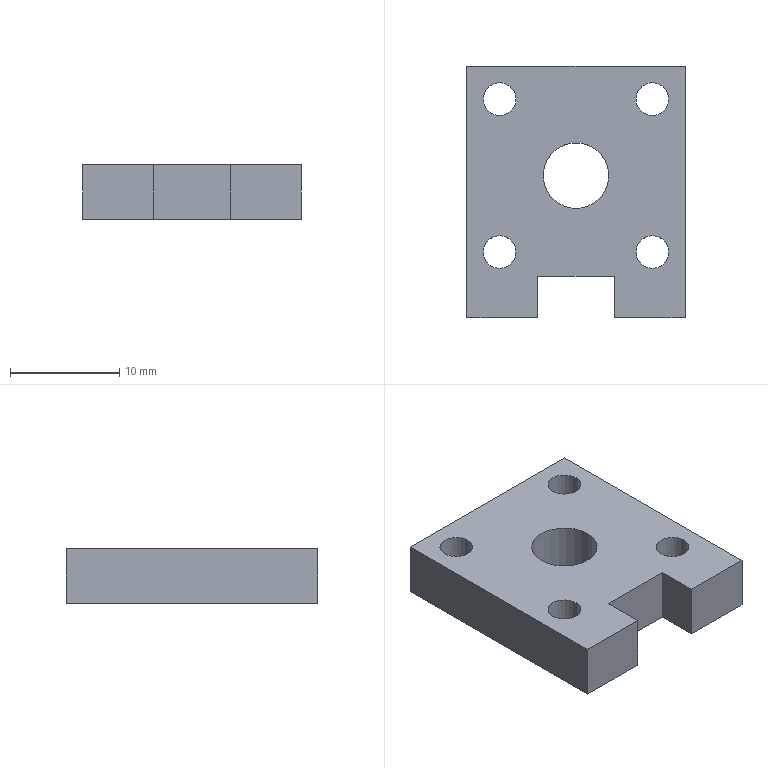Part | SolidWorks | features Extrusion 1 | 1 solid | 20 faces | box 20 x 23 x 5 mm | volume 1884 mm3 | cylinder 10 | plane 10 | commonest cylinder face diameters 3 x8 6 x2
STEP:
#1=CARTESIAN_POINT('',(-8.5,-7.,5.));
#2=VERTEX_POINT('',#1);
#3=CARTESIAN_POINT('',(-5.5,-7.,5.));
#4=VERTEX_POINT('',#3);
#5=CARTESIAN_POINT('',(-7.,-7.,5.));
#6=DIRECTION('',(0.,0.,1.));
#7=DIRECTION('',(1.,0.,0.));
#8=AXIS2_PLACEMENT_3D('',#5,#6,#7);
#9=CIRCLE('',#8,1.5);
#10=EDGE_CURVE('',#2,#4,#9,.T.);
#11=ORIENTED_EDGE('',*,*,#10,.T.);
#12=CARTESIAN_POINT('',(-5.5,-7.,0.));
#13=VERTEX_POINT('',#12);
#14=CARTESIAN_POINT('',(-5.5,-7.,5.));
#15=DIRECTION('',(0.,0.,-1.));
#16=VECTOR('',#15,1000.);
#17=LINE('',#14,#16);
#18=EDGE_CURVE('',#4,#13,#17,.T.);
#19=ORIENTED_EDGE('',*,*,#18,.T.);
#20=CARTESIAN_POINT('',(-8.5,-7.,0.));
#21=VERTEX_POINT('',#20);
#22=CARTESIAN_POINT('',(-7.,-7.,0.));
#23=DIRECTION('',(0.,0.,1.));
#24=DIRECTION('',(1.,0.,0.));
#25=AXIS2_PLACEMENT_3D('',#22,#23,#24);
#26=CIRCLE('',#25,1.5);
#27=EDGE_CURVE('',#21,#13,#26,.T.);
#28=ORIENTED_EDGE('',*,*,#27,.F.);
#29=CARTESIAN_POINT('',(-8.5,-7.,5.));
#30=DIRECTION('',(0.,0.,-1.));
#31=VECTOR('',#30,1000.);
#32=LINE('',#29,#31);
#33=EDGE_CURVE('',#2,#21,#32,.T.);
#34=ORIENTED_EDGE('',*,*,#33,.F.);
#35=EDGE_LOOP('',(#11,#19,#28,#34));
#36=FACE_OUTER_BOUND('',#35,.T.);
#37=CARTESIAN_POINT('',(-7.,-7.,5.));
#38=DIRECTION('',(0.,0.,-1.));
#39=DIRECTION('',(-1.,0.,0.));
#40=AXIS2_PLACEMENT_3D('',#37,#38,#39);
#41=CYLINDRICAL_SURFACE('',#40,1.5);
#42=ADVANCED_FACE('',(#36),#41,.F.);
#43=CARTESIAN_POINT('',(5.5,-7.,5.));
#44=VERTEX_POINT('',#43);
#45=CARTESIAN_POINT('',(8.5,-7.,5.));
#46=VERTEX_POINT('',#45);
#47=CARTESIAN_POINT('',(7.,-7.,5.));
#48=DIRECTION('',(0.,0.,1.));
#49=DIRECTION('',(1.,0.,0.));
#50=AXIS2_PLACEMENT_3D('',#47,#48,#49);
#51=CIRCLE('',#50,1.5);
#52=EDGE_CURVE('',#44,#46,#51,.T.);
#53=ORIENTED_EDGE('',*,*,#52,.T.);
#54=CARTESIAN_POINT('',(8.5,-7.,0.));
#55=VERTEX_POINT('',#54);
#56=CARTESIAN_POINT('',(8.5,-7.,5.));
#57=DIRECTION('',(0.,0.,-1.));
#58=VECTOR('',#57,1000.);
#59=LINE('',#56,#58);
#60=EDGE_CURVE('',#46,#55,#59,.T.);
#61=ORIENTED_EDGE('',*,*,#60,.T.);
#62=CARTESIAN_POINT('',(5.5,-7.,0.));
#63=VERTEX_POINT('',#62);
#64=CARTESIAN_POINT('',(7.,-7.,0.));
#65=DIRECTION('',(0.,0.,1.));
#66=DIRECTION('',(1.,0.,0.));
#67=AXIS2_PLACEMENT_3D('',#64,#65,#66);
#68=CIRCLE('',#67,1.5);
#69=EDGE_CURVE('',#63,#55,#68,.T.);
#70=ORIENTED_EDGE('',*,*,#69,.F.);
#71=CARTESIAN_POINT('',(5.5,-7.,5.));
#72=DIRECTION('',(0.,0.,-1.));
#73=VECTOR('',#72,1000.);
#74=LINE('',#71,#73);
#75=EDGE_CURVE('',#44,#63,#74,.T.);
#76=ORIENTED_EDGE('',*,*,#75,.F.);
#77=EDGE_LOOP('',(#53,#61,#70,#76));
#78=FACE_OUTER_BOUND('',#77,.T.);
#79=CARTESIAN_POINT('',(7.,-7.,5.));
#80=DIRECTION('',(0.,0.,-1.));
#81=DIRECTION('',(-1.,0.,0.));
#82=AXIS2_PLACEMENT_3D('',#79,#80,#81);
#83=CYLINDRICAL_SURFACE('',#82,1.5);
#84=ADVANCED_FACE('',(#78),#83,.F.);
#85=CARTESIAN_POINT('',(5.5,7.,5.));
#86=VERTEX_POINT('',#85);
#87=CARTESIAN_POINT('',(8.5,7.,5.));
#88=VERTEX_POINT('',#87);
#89=CARTESIAN_POINT('',(7.,7.,5.));
#90=DIRECTION('',(0.,0.,1.));
#91=DIRECTION('',(1.,0.,0.));
#92=AXIS2_PLACEMENT_3D('',#89,#90,#91);
#93=CIRCLE('',#92,1.5);
#94=EDGE_CURVE('',#86,#88,#93,.T.);
#95=ORIENTED_EDGE('',*,*,#94,.T.);
#96=CARTESIAN_POINT('',(8.5,7.,0.));
#97=VERTEX_POINT('',#96);
#98=CARTESIAN_POINT('',(8.5,7.,5.));
#99=DIRECTION('',(0.,0.,-1.));
#100=VECTOR('',#99,1000.);
#101=LINE('',#98,#100);
#102=EDGE_CURVE('',#88,#97,#101,.T.);
#103=ORIENTED_EDGE('',*,*,#102,.T.);
#104=CARTESIAN_POINT('',(5.5,7.,0.));
#105=VERTEX_POINT('',#104);
#106=CARTESIAN_POINT('',(7.,7.,0.));
#107=DIRECTION('',(0.,0.,1.));
#108=DIRECTION('',(1.,0.,0.));
#109=AXIS2_PLACEMENT_3D('',#106,#107,#108);
#110=CIRCLE('',#109,1.5);
#111=EDGE_CURVE('',#105,#97,#110,.T.);
#112=ORIENTED_EDGE('',*,*,#111,.F.);
#113=CARTESIAN_POINT('',(5.5,7.,5.));
#114=DIRECTION('',(0.,0.,-1.));
#115=VECTOR('',#114,1000.);
#116=LINE('',#113,#115);
#117=EDGE_CURVE('',#86,#105,#116,.T.);
#118=ORIENTED_EDGE('',*,*,#117,.F.);
#119=EDGE_LOOP('',(#95,#103,#112,#118));
#120=FACE_OUTER_BOUND('',#119,.T.);
#121=CARTESIAN_POINT('',(7.,7.,5.));
#122=DIRECTION('',(0.,0.,-1.));
#123=DIRECTION('',(-1.,0.,0.));
#124=AXIS2_PLACEMENT_3D('',#121,#122,#123);
#125=CYLINDRICAL_SURFACE('',#124,1.5);
#126=ADVANCED_FACE('',(#120),#125,.F.);
#127=CARTESIAN_POINT('',(-8.5,7.,5.));
#128=VERTEX_POINT('',#127);
#129=CARTESIAN_POINT('',(-5.5,7.,5.));
#130=VERTEX_POINT('',#129);
#131=CARTESIAN_POINT('',(-7.,7.,5.));
#132=DIRECTION('',(0.,0.,1.));
#133=DIRECTION('',(1.,0.,0.));
#134=AXIS2_PLACEMENT_3D('',#131,#132,#133);
#135=CIRCLE('',#134,1.5);
#136=EDGE_CURVE('',#128,#130,#135,.T.);
#137=ORIENTED_EDGE('',*,*,#136,.T.);
#138=CARTESIAN_POINT('',(-5.5,7.,0.));
#139=VERTEX_POINT('',#138);
#140=CARTESIAN_POINT('',(-5.5,7.,5.));
#141=DIRECTION('',(0.,0.,-1.));
#142=VECTOR('',#141,1000.);
#143=LINE('',#140,#142);
#144=EDGE_CURVE('',#130,#139,#143,.T.);
#145=ORIENTED_EDGE('',*,*,#144,.T.);
#146=CARTESIAN_POINT('',(-8.5,7.,0.));
#147=VERTEX_POINT('',#146);
#148=CARTESIAN_POINT('',(-7.,7.,0.));
#149=DIRECTION('',(0.,0.,1.));
#150=DIRECTION('',(1.,0.,0.));
#151=AXIS2_PLACEMENT_3D('',#148,#149,#150);
#152=CIRCLE('',#151,1.5);
#153=EDGE_CURVE('',#147,#139,#152,.T.);
#154=ORIENTED_EDGE('',*,*,#153,.F.);
#155=CARTESIAN_POINT('',(-8.5,7.,5.));
#156=DIRECTION('',(0.,0.,-1.));
#157=VECTOR('',#156,1000.);
#158=LINE('',#155,#157);
#159=EDGE_CURVE('',#128,#147,#158,.T.);
#160=ORIENTED_EDGE('',*,*,#159,.F.);
#161=EDGE_LOOP('',(#137,#145,#154,#160));
#162=FACE_OUTER_BOUND('',#161,.T.);
#163=CARTESIAN_POINT('',(-7.,7.,5.));
#164=DIRECTION('',(0.,0.,-1.));
#165=DIRECTION('',(-1.,0.,0.));
#166=AXIS2_PLACEMENT_3D('',#163,#164,#165);
#167=CYLINDRICAL_SURFACE('',#166,1.5);
#168=ADVANCED_FACE('',(#162),#167,.F.);
#169=CARTESIAN_POINT('',(-3.,0.,5.));
#170=VERTEX_POINT('',#169);
#171=CARTESIAN_POINT('',(3.,0.,5.));
#172=VERTEX_POINT('',#171);
#173=CARTESIAN_POINT('',(0.,0.,5.));
#174=DIRECTION('',(0.,0.,1.));
#175=DIRECTION('',(1.,0.,0.));
#176=AXIS2_PLACEMENT_3D('',#173,#174,#175);
#177=CIRCLE('',#176,3.);
#178=EDGE_CURVE('',#170,#172,#177,.T.);
#179=ORIENTED_EDGE('',*,*,#178,.T.);
#180=CARTESIAN_POINT('',(3.,0.,0.));
#181=VERTEX_POINT('',#180);
#182=CARTESIAN_POINT('',(3.,0.,5.));
#183=DIRECTION('',(0.,0.,-1.));
#184=VECTOR('',#183,1000.);
#185=LINE('',#182,#184);
#186=EDGE_CURVE('',#172,#181,#185,.T.);
#187=ORIENTED_EDGE('',*,*,#186,.T.);
#188=CARTESIAN_POINT('',(-3.,0.,0.));
#189=VERTEX_POINT('',#188);
#190=CARTESIAN_POINT('',(0.,0.,0.));
#191=DIRECTION('',(0.,0.,1.));
#192=DIRECTION('',(1.,0.,0.));
#193=AXIS2_PLACEMENT_3D('',#190,#191,#192);
#194=CIRCLE('',#193,3.);
#195=EDGE_CURVE('',#189,#181,#194,.T.);
#196=ORIENTED_EDGE('',*,*,#195,.F.);
#197=CARTESIAN_POINT('',(-3.,0.,5.));
#198=DIRECTION('',(0.,0.,-1.));
#199=VECTOR('',#198,1000.);
#200=LINE('',#197,#199);
#201=EDGE_CURVE('',#170,#189,#200,.T.);
#202=ORIENTED_EDGE('',*,*,#201,.F.);
#203=EDGE_LOOP('',(#179,#187,#196,#202));
#204=FACE_OUTER_BOUND('',#203,.T.);
#205=CARTESIAN_POINT('',(0.,0.,5.));
#206=DIRECTION('',(0.,0.,-1.));
#207=DIRECTION('',(-1.,0.,0.));
#208=AXIS2_PLACEMENT_3D('',#205,#206,#207);
#209=CYLINDRICAL_SURFACE('',#208,3.);
#210=ADVANCED_FACE('',(#204),#209,.F.);
#211=ORIENTED_EDGE('',*,*,#52,.F.);
#212=CARTESIAN_POINT('',(7.,-7.,5.));
#213=DIRECTION('',(0.,0.,1.));
#214=DIRECTION('',(1.,0.,0.));
#215=AXIS2_PLACEMENT_3D('',#212,#213,#214);
#216=CIRCLE('',#215,1.5);
#217=EDGE_CURVE('',#46,#44,#216,.T.);
#218=ORIENTED_EDGE('',*,*,#217,.F.);
#219=EDGE_LOOP('',(#211,#218));
#220=FACE_BOUND('',#219,.T.);
#221=ORIENTED_EDGE('',*,*,#136,.F.);
#222=CARTESIAN_POINT('',(-7.,7.,5.));
#223=DIRECTION('',(0.,0.,1.));
#224=DIRECTION('',(1.,0.,0.));
#225=AXIS2_PLACEMENT_3D('',#222,#223,#224);
#226=CIRCLE('',#225,1.5);
#227=EDGE_CURVE('',#130,#128,#226,.T.);
#228=ORIENTED_EDGE('',*,*,#227,.F.);
#229=EDGE_LOOP('',(#221,#228));
#230=FACE_BOUND('',#229,.T.);
#231=CARTESIAN_POINT('',(10.,10.,5.));
#232=VERTEX_POINT('',#231);
#233=CARTESIAN_POINT('',(-10.,10.,5.));
#234=VERTEX_POINT('',#233);
#235=CARTESIAN_POINT('',(5.,10.,5.));
#236=DIRECTION('',(-1.,0.,0.));
#237=VECTOR('',#236,1000.);
#238=LINE('',#235,#237);
#239=EDGE_CURVE('',#232,#234,#238,.T.);
#240=ORIENTED_EDGE('',*,*,#239,.T.);
#241=CARTESIAN_POINT('',(-10.,-13.,5.));
#242=VERTEX_POINT('',#241);
#243=CARTESIAN_POINT('',(-10.,-10.,5.));
#244=DIRECTION('',(0.,-1.,0.));
#245=VECTOR('',#244,1000.);
#246=LINE('',#243,#245);
#247=EDGE_CURVE('',#234,#242,#246,.T.);
#248=ORIENTED_EDGE('',*,*,#247,.T.);
#249=CARTESIAN_POINT('',(-3.5,-13.,5.));
#250=VERTEX_POINT('',#249);
#251=CARTESIAN_POINT('',(-3.5,-13.,5.));
#252=DIRECTION('',(1.,0.,0.));
#253=VECTOR('',#252,1000.);
#254=LINE('',#251,#253);
#255=EDGE_CURVE('',#242,#250,#254,.T.);
#256=ORIENTED_EDGE('',*,*,#255,.T.);
#257=CARTESIAN_POINT('',(-3.5,-9.2,5.));
#258=VERTEX_POINT('',#257);
#259=CARTESIAN_POINT('',(-3.5,-9.2,5.));
#260=DIRECTION('',(0.,1.,0.));
#261=VECTOR('',#260,1000.);
#262=LINE('',#259,#261);
#263=EDGE_CURVE('',#250,#258,#262,.T.);
#264=ORIENTED_EDGE('',*,*,#263,.T.);
#265=CARTESIAN_POINT('',(3.5,-9.2,5.));
#266=VERTEX_POINT('',#265);
#267=CARTESIAN_POINT('',(3.5,-9.2,5.));
#268=DIRECTION('',(1.,0.,0.));
#269=VECTOR('',#268,1000.);
#270=LINE('',#267,#269);
#271=EDGE_CURVE('',#258,#266,#270,.T.);
#272=ORIENTED_EDGE('',*,*,#271,.T.);
#273=CARTESIAN_POINT('',(3.5,-13.,5.));
#274=VERTEX_POINT('',#273);
#275=CARTESIAN_POINT('',(3.5,-13.,5.));
#276=DIRECTION('',(0.,-1.,0.));
#277=VECTOR('',#276,1000.);
#278=LINE('',#275,#277);
#279=EDGE_CURVE('',#266,#274,#278,.T.);
#280=ORIENTED_EDGE('',*,*,#279,.T.);
#281=CARTESIAN_POINT('',(10.,-13.,5.));
#282=VERTEX_POINT('',#281);
#283=CARTESIAN_POINT('',(10.,-13.,5.));
#284=DIRECTION('',(1.,0.,0.));
#285=VECTOR('',#284,1000.);
#286=LINE('',#283,#285);
#287=EDGE_CURVE('',#274,#282,#286,.T.);
#288=ORIENTED_EDGE('',*,*,#287,.T.);
#289=CARTESIAN_POINT('',(10.,-10.,5.));
#290=DIRECTION('',(0.,1.,0.));
#291=VECTOR('',#290,1000.);
#292=LINE('',#289,#291);
#293=EDGE_CURVE('',#282,#232,#292,.T.);
#294=ORIENTED_EDGE('',*,*,#293,.T.);
#295=EDGE_LOOP('',(#240,#248,#256,#264,#272,#280,#288,#294));
#296=FACE_OUTER_BOUND('',#295,.T.);
#297=ORIENTED_EDGE('',*,*,#178,.F.);
#298=CARTESIAN_POINT('',(0.,0.,5.));
#299=DIRECTION('',(0.,0.,1.));
#300=DIRECTION('',(1.,0.,0.));
#301=AXIS2_PLACEMENT_3D('',#298,#299,#300);
#302=CIRCLE('',#301,3.);
#303=EDGE_CURVE('',#172,#170,#302,.T.);
#304=ORIENTED_EDGE('',*,*,#303,.F.);
#305=EDGE_LOOP('',(#297,#304));
#306=FACE_BOUND('',#305,.T.);
#307=ORIENTED_EDGE('',*,*,#94,.F.);
#308=CARTESIAN_POINT('',(7.,7.,5.));
#309=DIRECTION('',(0.,0.,1.));
#310=DIRECTION('',(1.,0.,0.));
#311=AXIS2_PLACEMENT_3D('',#308,#309,#310);
#312=CIRCLE('',#311,1.5);
#313=EDGE_CURVE('',#88,#86,#312,.T.);
#314=ORIENTED_EDGE('',*,*,#313,.F.);
#315=EDGE_LOOP('',(#307,#314));
#316=FACE_BOUND('',#315,.T.);
#317=ORIENTED_EDGE('',*,*,#10,.F.);
#318=CARTESIAN_POINT('',(-7.,-7.,5.));
#319=DIRECTION('',(0.,0.,1.));
#320=DIRECTION('',(1.,0.,0.));
#321=AXIS2_PLACEMENT_3D('',#318,#319,#320);
#322=CIRCLE('',#321,1.5);
#323=EDGE_CURVE('',#4,#2,#322,.T.);
#324=ORIENTED_EDGE('',*,*,#323,.F.);
#325=EDGE_LOOP('',(#317,#324));
#326=FACE_BOUND('',#325,.T.);
#327=CARTESIAN_POINT('',(0.,0.,5.));
#328=DIRECTION('',(0.,0.,1.));
#329=DIRECTION('',(1.,0.,0.));
#330=AXIS2_PLACEMENT_3D('',#327,#328,#329);
#331=PLANE('',#330);
#332=ADVANCED_FACE('',(#220,#230,#296,#306,#316,#326),#331,.T.);
#333=CARTESIAN_POINT('',(10.,10.,0.));
#334=VERTEX_POINT('',#333);
#335=CARTESIAN_POINT('',(-10.,10.,0.));
#336=VERTEX_POINT('',#335);
#337=CARTESIAN_POINT('',(-10.,10.,0.));
#338=DIRECTION('',(-1.,0.,0.));
#339=VECTOR('',#338,1000.);
#340=LINE('',#337,#339);
#341=EDGE_CURVE('',#334,#336,#340,.T.);
#342=ORIENTED_EDGE('',*,*,#341,.F.);
#343=CARTESIAN_POINT('',(10.,-13.,0.));
#344=VERTEX_POINT('',#343);
#345=CARTESIAN_POINT('',(10.,-10.,0.));
#346=DIRECTION('',(0.,1.,0.));
#347=VECTOR('',#346,1000.);
#348=LINE('',#345,#347);
#349=EDGE_CURVE('',#344,#334,#348,.T.);
#350=ORIENTED_EDGE('',*,*,#349,.F.);
#351=CARTESIAN_POINT('',(3.5,-13.,0.));
#352=VERTEX_POINT('',#351);
#353=CARTESIAN_POINT('',(10.,-13.,0.));
#354=DIRECTION('',(1.,0.,0.));
#355=VECTOR('',#354,1000.);
#356=LINE('',#353,#355);
#357=EDGE_CURVE('',#352,#344,#356,.T.);
#358=ORIENTED_EDGE('',*,*,#357,.F.);
#359=CARTESIAN_POINT('',(3.5,-9.2,0.));
#360=VERTEX_POINT('',#359);
#361=CARTESIAN_POINT('',(3.5,-13.,0.));
#362=DIRECTION('',(0.,-1.,0.));
#363=VECTOR('',#362,1000.);
#364=LINE('',#361,#363);
#365=EDGE_CURVE('',#360,#352,#364,.T.);
#366=ORIENTED_EDGE('',*,*,#365,.F.);
#367=CARTESIAN_POINT('',(-3.5,-9.2,0.));
#368=VERTEX_POINT('',#367);
#369=CARTESIAN_POINT('',(3.5,-9.2,0.));
#370=DIRECTION('',(1.,0.,0.));
#371=VECTOR('',#370,1000.);
#372=LINE('',#369,#371);
#373=EDGE_CURVE('',#368,#360,#372,.T.);
#374=ORIENTED_EDGE('',*,*,#373,.F.);
#375=CARTESIAN_POINT('',(-3.5,-13.,0.));
#376=VERTEX_POINT('',#375);
#377=CARTESIAN_POINT('',(-3.5,-9.2,0.));
#378=DIRECTION('',(0.,1.,0.));
#379=VECTOR('',#378,1000.);
#380=LINE('',#377,#379);
#381=EDGE_CURVE('',#376,#368,#380,.T.);
#382=ORIENTED_EDGE('',*,*,#381,.F.);
#383=CARTESIAN_POINT('',(-10.,-13.,0.));
#384=VERTEX_POINT('',#383);
#385=CARTESIAN_POINT('',(-3.5,-13.,0.));
#386=DIRECTION('',(1.,0.,0.));
#387=VECTOR('',#386,1000.);
#388=LINE('',#385,#387);
#389=EDGE_CURVE('',#384,#376,#388,.T.);
#390=ORIENTED_EDGE('',*,*,#389,.F.);
#391=CARTESIAN_POINT('',(-10.,-10.,0.));
#392=DIRECTION('',(0.,-1.,0.));
#393=VECTOR('',#392,1000.);
#394=LINE('',#391,#393);
#395=EDGE_CURVE('',#336,#384,#394,.T.);
#396=ORIENTED_EDGE('',*,*,#395,.F.);
#397=EDGE_LOOP('',(#342,#350,#358,#366,#374,#382,#390,#396));
#398=FACE_OUTER_BOUND('',#397,.T.);
#399=ORIENTED_EDGE('',*,*,#195,.T.);
#400=CARTESIAN_POINT('',(0.,0.,0.));
#401=DIRECTION('',(0.,0.,1.));
#402=DIRECTION('',(1.,0.,0.));
#403=AXIS2_PLACEMENT_3D('',#400,#401,#402);
#404=CIRCLE('',#403,3.);
#405=EDGE_CURVE('',#181,#189,#404,.T.);
#406=ORIENTED_EDGE('',*,*,#405,.T.);
#407=EDGE_LOOP('',(#399,#406));
#408=FACE_BOUND('',#407,.T.);
#409=ORIENTED_EDGE('',*,*,#153,.T.);
#410=CARTESIAN_POINT('',(-7.,7.,0.));
#411=DIRECTION('',(0.,0.,1.));
#412=DIRECTION('',(1.,0.,0.));
#413=AXIS2_PLACEMENT_3D('',#410,#411,#412);
#414=CIRCLE('',#413,1.5);
#415=EDGE_CURVE('',#139,#147,#414,.T.);
#416=ORIENTED_EDGE('',*,*,#415,.T.);
#417=EDGE_LOOP('',(#409,#416));
#418=FACE_BOUND('',#417,.T.);
#419=ORIENTED_EDGE('',*,*,#111,.T.);
#420=CARTESIAN_POINT('',(7.,7.,0.));
#421=DIRECTION('',(0.,0.,1.));
#422=DIRECTION('',(1.,0.,0.));
#423=AXIS2_PLACEMENT_3D('',#420,#421,#422);
#424=CIRCLE('',#423,1.5);
#425=EDGE_CURVE('',#97,#105,#424,.T.);
#426=ORIENTED_EDGE('',*,*,#425,.T.);
#427=EDGE_LOOP('',(#419,#426));
#428=FACE_BOUND('',#427,.T.);
#429=ORIENTED_EDGE('',*,*,#69,.T.);
#430=CARTESIAN_POINT('',(7.,-7.,0.));
#431=DIRECTION('',(0.,0.,1.));
#432=DIRECTION('',(1.,0.,0.));
#433=AXIS2_PLACEMENT_3D('',#430,#431,#432);
#434=CIRCLE('',#433,1.5);
#435=EDGE_CURVE('',#55,#63,#434,.T.);
#436=ORIENTED_EDGE('',*,*,#435,.T.);
#437=EDGE_LOOP('',(#429,#436));
#438=FACE_BOUND('',#437,.T.);
#439=ORIENTED_EDGE('',*,*,#27,.T.);
#440=CARTESIAN_POINT('',(-7.,-7.,0.));
#441=DIRECTION('',(0.,0.,1.));
#442=DIRECTION('',(1.,0.,0.));
#443=AXIS2_PLACEMENT_3D('',#440,#441,#442);
#444=CIRCLE('',#443,1.5);
#445=EDGE_CURVE('',#13,#21,#444,.T.);
#446=ORIENTED_EDGE('',*,*,#445,.T.);
#447=EDGE_LOOP('',(#439,#446));
#448=FACE_BOUND('',#447,.T.);
#449=CARTESIAN_POINT('',(0.,0.,0.));
#450=DIRECTION('',(0.,0.,1.));
#451=DIRECTION('',(1.,0.,0.));
#452=AXIS2_PLACEMENT_3D('',#449,#450,#451);
#453=PLANE('',#452);
#454=ADVANCED_FACE('',(#398,#408,#418,#428,#438,#448),#453,.F.);
#455=ORIENTED_EDGE('',*,*,#341,.T.);
#456=CARTESIAN_POINT('',(-10.,10.,5.));
#457=DIRECTION('',(0.,0.,-1.));
#458=VECTOR('',#457,1000.);
#459=LINE('',#456,#458);
#460=EDGE_CURVE('',#234,#336,#459,.T.);
#461=ORIENTED_EDGE('',*,*,#460,.F.);
#462=ORIENTED_EDGE('',*,*,#239,.F.);
#463=CARTESIAN_POINT('',(10.,10.,5.));
#464=DIRECTION('',(0.,0.,-1.));
#465=VECTOR('',#464,1000.);
#466=LINE('',#463,#465);
#467=EDGE_CURVE('',#232,#334,#466,.T.);
#468=ORIENTED_EDGE('',*,*,#467,.T.);
#469=EDGE_LOOP('',(#455,#461,#462,#468));
#470=FACE_OUTER_BOUND('',#469,.T.);
#471=CARTESIAN_POINT('',(-10.,10.,5.));
#472=DIRECTION('',(0.,-1.,0.));
#473=DIRECTION('',(1.,0.,0.));
#474=AXIS2_PLACEMENT_3D('',#471,#472,#473);
#475=PLANE('',#474);
#476=ADVANCED_FACE('',(#470),#475,.F.);
#477=ORIENTED_EDGE('',*,*,#395,.T.);
#478=CARTESIAN_POINT('',(-10.,-13.,5.));
#479=DIRECTION('',(0.,0.,-1.));
#480=VECTOR('',#479,1000.);
#481=LINE('',#478,#480);
#482=EDGE_CURVE('',#242,#384,#481,.T.);
#483=ORIENTED_EDGE('',*,*,#482,.F.);
#484=ORIENTED_EDGE('',*,*,#247,.F.);
#485=ORIENTED_EDGE('',*,*,#460,.T.);
#486=EDGE_LOOP('',(#477,#483,#484,#485));
#487=FACE_OUTER_BOUND('',#486,.T.);
#488=CARTESIAN_POINT('',(-10.,-10.,5.));
#489=DIRECTION('',(1.,0.,0.));
#490=DIRECTION('',(0.,0.,-1.));
#491=AXIS2_PLACEMENT_3D('',#488,#489,#490);
#492=PLANE('',#491);
#493=ADVANCED_FACE('',(#487),#492,.F.);
#494=ORIENTED_EDGE('',*,*,#389,.T.);
#495=CARTESIAN_POINT('',(-3.5,-13.,5.));
#496=DIRECTION('',(0.,0.,-1.));
#497=VECTOR('',#496,1000.);
#498=LINE('',#495,#497);
#499=EDGE_CURVE('',#250,#376,#498,.T.);
#500=ORIENTED_EDGE('',*,*,#499,.F.);
#501=ORIENTED_EDGE('',*,*,#255,.F.);
#502=ORIENTED_EDGE('',*,*,#482,.T.);
#503=EDGE_LOOP('',(#494,#500,#501,#502));
#504=FACE_OUTER_BOUND('',#503,.T.);
#505=CARTESIAN_POINT('',(-3.5,-13.,5.));
#506=DIRECTION('',(0.,1.,0.));
#507=DIRECTION('',(0.,0.,1.));
#508=AXIS2_PLACEMENT_3D('',#505,#506,#507);
#509=PLANE('',#508);
#510=ADVANCED_FACE('',(#504),#509,.F.);
#511=ORIENTED_EDGE('',*,*,#381,.T.);
#512=CARTESIAN_POINT('',(-3.5,-9.2,5.));
#513=DIRECTION('',(0.,0.,-1.));
#514=VECTOR('',#513,1000.);
#515=LINE('',#512,#514);
#516=EDGE_CURVE('',#258,#368,#515,.T.);
#517=ORIENTED_EDGE('',*,*,#516,.F.);
#518=ORIENTED_EDGE('',*,*,#263,.F.);
#519=ORIENTED_EDGE('',*,*,#499,.T.);
#520=EDGE_LOOP('',(#511,#517,#518,#519));
#521=FACE_OUTER_BOUND('',#520,.T.);
#522=CARTESIAN_POINT('',(-3.5,-9.2,5.));
#523=DIRECTION('',(-1.,0.,0.));
#524=DIRECTION('',(0.,-1.,0.));
#525=AXIS2_PLACEMENT_3D('',#522,#523,#524);
#526=PLANE('',#525);
#527=ADVANCED_FACE('',(#521),#526,.F.);
#528=ORIENTED_EDGE('',*,*,#373,.T.);
#529=CARTESIAN_POINT('',(3.5,-9.2,5.));
#530=DIRECTION('',(0.,0.,-1.));
#531=VECTOR('',#530,1000.);
#532=LINE('',#529,#531);
#533=EDGE_CURVE('',#266,#360,#532,.T.);
#534=ORIENTED_EDGE('',*,*,#533,.F.);
#535=ORIENTED_EDGE('',*,*,#271,.F.);
#536=ORIENTED_EDGE('',*,*,#516,.T.);
#537=EDGE_LOOP('',(#528,#534,#535,#536));
#538=FACE_OUTER_BOUND('',#537,.T.);
#539=CARTESIAN_POINT('',(3.5,-9.2,5.));
#540=DIRECTION('',(0.,1.,0.));
#541=DIRECTION('',(0.,0.,1.));
#542=AXIS2_PLACEMENT_3D('',#539,#540,#541);
#543=PLANE('',#542);
#544=ADVANCED_FACE('',(#538),#543,.F.);
#545=ORIENTED_EDGE('',*,*,#365,.T.);
#546=CARTESIAN_POINT('',(3.5,-13.,5.));
#547=DIRECTION('',(0.,0.,-1.));
#548=VECTOR('',#547,1000.);
#549=LINE('',#546,#548);
#550=EDGE_CURVE('',#274,#352,#549,.T.);
#551=ORIENTED_EDGE('',*,*,#550,.F.);
#552=ORIENTED_EDGE('',*,*,#279,.F.);
#553=ORIENTED_EDGE('',*,*,#533,.T.);
#554=EDGE_LOOP('',(#545,#551,#552,#553));
#555=FACE_OUTER_BOUND('',#554,.T.);
#556=CARTESIAN_POINT('',(3.5,-13.,5.));
#557=DIRECTION('',(1.,0.,0.));
#558=DIRECTION('',(0.,0.,-1.));
#559=AXIS2_PLACEMENT_3D('',#556,#557,#558);
#560=PLANE('',#559);
#561=ADVANCED_FACE('',(#555),#560,.F.);
#562=ORIENTED_EDGE('',*,*,#357,.T.);
#563=CARTESIAN_POINT('',(10.,-13.,5.));
#564=DIRECTION('',(0.,0.,-1.));
#565=VECTOR('',#564,1000.);
#566=LINE('',#563,#565);
#567=EDGE_CURVE('',#282,#344,#566,.T.);
#568=ORIENTED_EDGE('',*,*,#567,.F.);
#569=ORIENTED_EDGE('',*,*,#287,.F.);
#570=ORIENTED_EDGE('',*,*,#550,.T.);
#571=EDGE_LOOP('',(#562,#568,#569,#570));
#572=FACE_OUTER_BOUND('',#571,.T.);
#573=CARTESIAN_POINT('',(10.,-13.,5.));
#574=DIRECTION('',(0.,1.,0.));
#575=DIRECTION('',(0.,0.,1.));
#576=AXIS2_PLACEMENT_3D('',#573,#574,#575);
#577=PLANE('',#576);
#578=ADVANCED_FACE('',(#572),#577,.F.);
#579=ORIENTED_EDGE('',*,*,#349,.T.);
#580=ORIENTED_EDGE('',*,*,#467,.F.);
#581=ORIENTED_EDGE('',*,*,#293,.F.);
#582=ORIENTED_EDGE('',*,*,#567,.T.);
#583=EDGE_LOOP('',(#579,#580,#581,#582));
#584=FACE_OUTER_BOUND('',#583,.T.);
#585=CARTESIAN_POINT('',(10.,-10.,5.));
#586=DIRECTION('',(-1.,0.,0.));
#587=DIRECTION('',(0.,0.,1.));
#588=AXIS2_PLACEMENT_3D('',#585,#586,#587);
#589=PLANE('',#588);
#590=ADVANCED_FACE('',(#584),#589,.F.);
#591=ORIENTED_EDGE('',*,*,#186,.F.);
#592=ORIENTED_EDGE('',*,*,#303,.T.);
#593=ORIENTED_EDGE('',*,*,#201,.T.);
#594=ORIENTED_EDGE('',*,*,#405,.F.);
#595=EDGE_LOOP('',(#591,#592,#593,#594));
#596=FACE_OUTER_BOUND('',#595,.T.);
#597=CARTESIAN_POINT('',(0.,0.,5.));
#598=DIRECTION('',(0.,0.,-1.));
#599=DIRECTION('',(-1.,0.,0.));
#600=AXIS2_PLACEMENT_3D('',#597,#598,#599);
#601=CYLINDRICAL_SURFACE('',#600,3.);
#602=ADVANCED_FACE('',(#596),#601,.F.);
#603=ORIENTED_EDGE('',*,*,#144,.F.);
#604=ORIENTED_EDGE('',*,*,#227,.T.);
#605=ORIENTED_EDGE('',*,*,#159,.T.);
#606=ORIENTED_EDGE('',*,*,#415,.F.);
#607=EDGE_LOOP('',(#603,#604,#605,#606));
#608=FACE_OUTER_BOUND('',#607,.T.);
#609=CARTESIAN_POINT('',(-7.,7.,5.));
#610=DIRECTION('',(0.,0.,-1.));
#611=DIRECTION('',(-1.,0.,0.));
#612=AXIS2_PLACEMENT_3D('',#609,#610,#611);
#613=CYLINDRICAL_SURFACE('',#612,1.5);
#614=ADVANCED_FACE('',(#608),#613,.F.);
#615=ORIENTED_EDGE('',*,*,#102,.F.);
#616=ORIENTED_EDGE('',*,*,#313,.T.);
#617=ORIENTED_EDGE('',*,*,#117,.T.);
#618=ORIENTED_EDGE('',*,*,#425,.F.);
#619=EDGE_LOOP('',(#615,#616,#617,#618));
#620=FACE_OUTER_BOUND('',#619,.T.);
#621=CARTESIAN_POINT('',(7.,7.,5.));
#622=DIRECTION('',(0.,0.,-1.));
#623=DIRECTION('',(-1.,0.,0.));
#624=AXIS2_PLACEMENT_3D('',#621,#622,#623);
#625=CYLINDRICAL_SURFACE('',#624,1.5);
#626=ADVANCED_FACE('',(#620),#625,.F.);
#627=ORIENTED_EDGE('',*,*,#60,.F.);
#628=ORIENTED_EDGE('',*,*,#217,.T.);
#629=ORIENTED_EDGE('',*,*,#75,.T.);
#630=ORIENTED_EDGE('',*,*,#435,.F.);
#631=EDGE_LOOP('',(#627,#628,#629,#630));
#632=FACE_OUTER_BOUND('',#631,.T.);
#633=CARTESIAN_POINT('',(7.,-7.,5.));
#634=DIRECTION('',(0.,0.,-1.));
#635=DIRECTION('',(-1.,0.,0.));
#636=AXIS2_PLACEMENT_3D('',#633,#634,#635);
#637=CYLINDRICAL_SURFACE('',#636,1.5);
#638=ADVANCED_FACE('',(#632),#637,.F.);
#639=ORIENTED_EDGE('',*,*,#18,.F.);
#640=ORIENTED_EDGE('',*,*,#323,.T.);
#641=ORIENTED_EDGE('',*,*,#33,.T.);
#642=ORIENTED_EDGE('',*,*,#445,.F.);
#643=EDGE_LOOP('',(#639,#640,#641,#642));
#644=FACE_OUTER_BOUND('',#643,.T.);
#645=CARTESIAN_POINT('',(-7.,-7.,5.));
#646=DIRECTION('',(0.,0.,-1.));
#647=DIRECTION('',(-1.,0.,0.));
#648=AXIS2_PLACEMENT_3D('',#645,#646,#647);
#649=CYLINDRICAL_SURFACE('',#648,1.5);
#650=ADVANCED_FACE('',(#644),#649,.F.);
#651=CLOSED_SHELL('',(#42,#84,#126,#168,#210,#332,#454,#476,#493,#510,#527,#544,#561,#578,#590,#602,#614,#626,#638,#650));
#652=MANIFOLD_SOLID_BREP('',#651);
#653=CARTESIAN_POINT('',(0.,0.,0.));
#654=DIRECTION('',(0.,0.,1.));
#655=DIRECTION('',(1.,0.,0.));
#656=AXIS2_PLACEMENT_3D('',#653,#654,#655);
#657=(LENGTH_UNIT()NAMED_UNIT(*)SI_UNIT(.MILLI.,.METRE.));
#658=UNCERTAINTY_MEASURE_WITH_UNIT(LENGTH_MEASURE(0.00001),#657,'','');
#659=(NAMED_UNIT(*)PLANE_ANGLE_UNIT()SI_UNIT($,.RADIAN.));
#660=(NAMED_UNIT(*)SI_UNIT($,.STERADIAN.)SOLID_ANGLE_UNIT());
#661=(GEOMETRIC_REPRESENTATION_CONTEXT(3)GLOBAL_UNCERTAINTY_ASSIGNED_CONTEXT((#658))GLOBAL_UNIT_ASSIGNED_CONTEXT((#657,#659,#660))REPRESENTATION_CONTEXT('',''));
#662=ADVANCED_BREP_SHAPE_REPRESENTATION('',(#652,#656),#661);